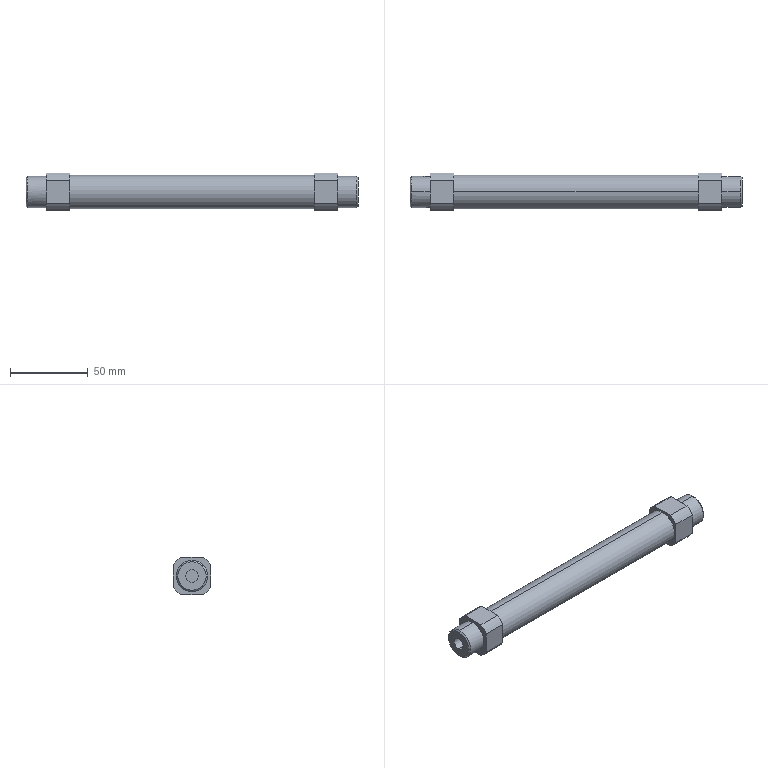Part | STEP file | _CDM2L20-75SZ-M9NW(0)_BODY | 1 solid | 49 faces | box 213 x 24 x 24 mm | volume 52685 mm3 | cylinder 22 | plane 17 | cone 10 | commonest cylinder face diameters 28 x8 20 x6 8.566 x4 8 x2 21.6 x2